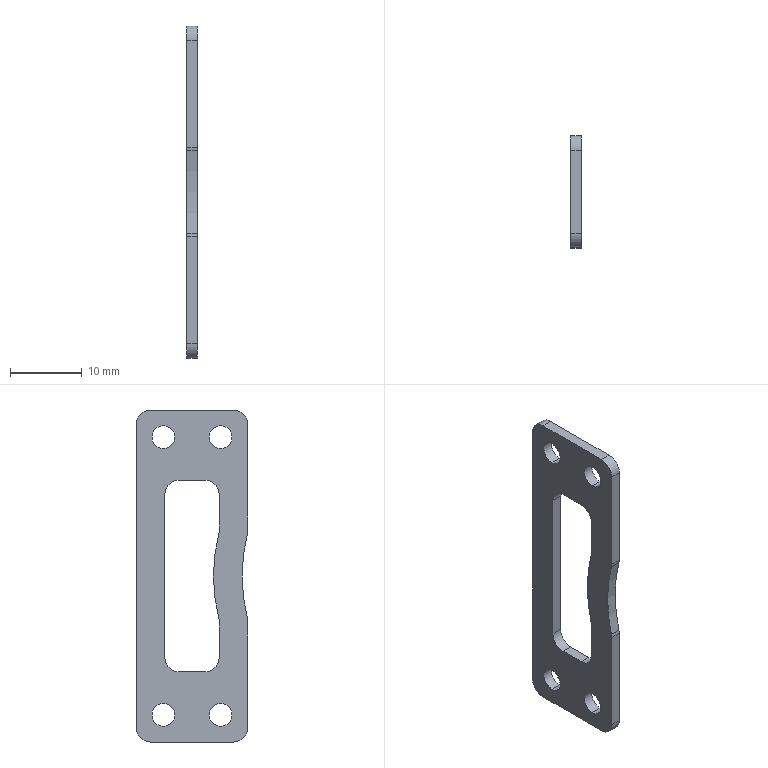Part | SolidWorks | features ICE 2, Extrusion 1, Fillet 1 | 1 solid | 34 faces | box 1.5 x 15.6 x 46.4 mm | volume 731.985 mm3 | cylinder 22 | plane 12 | commonest cylinder face diameters 4 x12 3.2 x8 46 x2
STEP:
#1=CARTESIAN_POINT('',(1.5,-8.,-37.2));
#2=VERTEX_POINT('',#1);
#3=CARTESIAN_POINT('',(1.5,-8.,-40.4));
#4=VERTEX_POINT('',#3);
#5=CARTESIAN_POINT('',(1.5,-8.,-38.8));
#6=DIRECTION('',(1.,0.,0.));
#7=DIRECTION('',(0.,0.,-1.));
#8=AXIS2_PLACEMENT_3D('',#5,#6,#7);
#9=CIRCLE('',#8,1.6);
#10=EDGE_CURVE('',#2,#4,#9,.T.);
#11=ORIENTED_EDGE('',*,*,#10,.T.);
#12=CARTESIAN_POINT('',(0.,-8.,-40.4));
#13=VERTEX_POINT('',#12);
#14=CARTESIAN_POINT('',(1.5,-8.,-40.4));
#15=DIRECTION('',(-1.,0.,0.));
#16=VECTOR('',#15,1000.);
#17=LINE('',#14,#16);
#18=EDGE_CURVE('',#4,#13,#17,.T.);
#19=ORIENTED_EDGE('',*,*,#18,.T.);
#20=CARTESIAN_POINT('',(0.,-8.,-37.2));
#21=VERTEX_POINT('',#20);
#22=CARTESIAN_POINT('',(0.,-8.,-38.8));
#23=DIRECTION('',(1.,0.,0.));
#24=DIRECTION('',(0.,0.,-1.));
#25=AXIS2_PLACEMENT_3D('',#22,#23,#24);
#26=CIRCLE('',#25,1.6);
#27=EDGE_CURVE('',#21,#13,#26,.T.);
#28=ORIENTED_EDGE('',*,*,#27,.F.);
#29=CARTESIAN_POINT('',(1.5,-8.,-37.2));
#30=DIRECTION('',(-1.,0.,0.));
#31=VECTOR('',#30,1000.);
#32=LINE('',#29,#31);
#33=EDGE_CURVE('',#2,#21,#32,.T.);
#34=ORIENTED_EDGE('',*,*,#33,.F.);
#35=EDGE_LOOP('',(#11,#19,#28,#34));
#36=FACE_OUTER_BOUND('',#35,.T.);
#37=CARTESIAN_POINT('',(1.5,-8.,-38.8));
#38=DIRECTION('',(-1.,0.,0.));
#39=DIRECTION('',(0.,0.,1.));
#40=AXIS2_PLACEMENT_3D('',#37,#38,#39);
#41=CYLINDRICAL_SURFACE('',#40,1.6);
#42=ADVANCED_FACE('',(#36),#41,.F.);
#43=CARTESIAN_POINT('',(1.5,0.,-37.2));
#44=VERTEX_POINT('',#43);
#45=CARTESIAN_POINT('',(1.5,0.,-40.4));
#46=VERTEX_POINT('',#45);
#47=CARTESIAN_POINT('',(1.5,0.,-38.8));
#48=DIRECTION('',(1.,0.,0.));
#49=DIRECTION('',(0.,0.,-1.));
#50=AXIS2_PLACEMENT_3D('',#47,#48,#49);
#51=CIRCLE('',#50,1.6);
#52=EDGE_CURVE('',#44,#46,#51,.T.);
#53=ORIENTED_EDGE('',*,*,#52,.T.);
#54=CARTESIAN_POINT('',(0.,0.,-40.4));
#55=VERTEX_POINT('',#54);
#56=CARTESIAN_POINT('',(1.5,0.,-40.4));
#57=DIRECTION('',(-1.,0.,0.));
#58=VECTOR('',#57,1000.);
#59=LINE('',#56,#58);
#60=EDGE_CURVE('',#46,#55,#59,.T.);
#61=ORIENTED_EDGE('',*,*,#60,.T.);
#62=CARTESIAN_POINT('',(0.,0.,-37.2));
#63=VERTEX_POINT('',#62);
#64=CARTESIAN_POINT('',(0.,0.,-38.8));
#65=DIRECTION('',(1.,0.,0.));
#66=DIRECTION('',(0.,0.,-1.));
#67=AXIS2_PLACEMENT_3D('',#64,#65,#66);
#68=CIRCLE('',#67,1.6);
#69=EDGE_CURVE('',#63,#55,#68,.T.);
#70=ORIENTED_EDGE('',*,*,#69,.F.);
#71=CARTESIAN_POINT('',(1.5,0.,-37.2));
#72=DIRECTION('',(-1.,0.,0.));
#73=VECTOR('',#72,1000.);
#74=LINE('',#71,#73);
#75=EDGE_CURVE('',#44,#63,#74,.T.);
#76=ORIENTED_EDGE('',*,*,#75,.F.);
#77=EDGE_LOOP('',(#53,#61,#70,#76));
#78=FACE_OUTER_BOUND('',#77,.T.);
#79=CARTESIAN_POINT('',(1.5,0.,-38.8));
#80=DIRECTION('',(-1.,0.,0.));
#81=DIRECTION('',(0.,0.,1.));
#82=AXIS2_PLACEMENT_3D('',#79,#80,#81);
#83=CYLINDRICAL_SURFACE('',#82,1.6);
#84=ADVANCED_FACE('',(#78),#83,.F.);
#85=CARTESIAN_POINT('',(1.5,-8.,1.6));
#86=VERTEX_POINT('',#85);
#87=CARTESIAN_POINT('',(1.5,-8.,-1.6));
#88=VERTEX_POINT('',#87);
#89=CARTESIAN_POINT('',(1.5,-8.,0.));
#90=DIRECTION('',(1.,0.,0.));
#91=DIRECTION('',(0.,0.,-1.));
#92=AXIS2_PLACEMENT_3D('',#89,#90,#91);
#93=CIRCLE('',#92,1.6);
#94=EDGE_CURVE('',#86,#88,#93,.T.);
#95=ORIENTED_EDGE('',*,*,#94,.T.);
#96=CARTESIAN_POINT('',(0.,-8.,-1.6));
#97=VERTEX_POINT('',#96);
#98=CARTESIAN_POINT('',(1.5,-8.,-1.6));
#99=DIRECTION('',(-1.,0.,0.));
#100=VECTOR('',#99,1000.);
#101=LINE('',#98,#100);
#102=EDGE_CURVE('',#88,#97,#101,.T.);
#103=ORIENTED_EDGE('',*,*,#102,.T.);
#104=CARTESIAN_POINT('',(0.,-8.,1.6));
#105=VERTEX_POINT('',#104);
#106=CARTESIAN_POINT('',(0.,-8.,0.));
#107=DIRECTION('',(1.,0.,0.));
#108=DIRECTION('',(0.,0.,-1.));
#109=AXIS2_PLACEMENT_3D('',#106,#107,#108);
#110=CIRCLE('',#109,1.6);
#111=EDGE_CURVE('',#105,#97,#110,.T.);
#112=ORIENTED_EDGE('',*,*,#111,.F.);
#113=CARTESIAN_POINT('',(1.5,-8.,1.6));
#114=DIRECTION('',(-1.,0.,0.));
#115=VECTOR('',#114,1000.);
#116=LINE('',#113,#115);
#117=EDGE_CURVE('',#86,#105,#116,.T.);
#118=ORIENTED_EDGE('',*,*,#117,.F.);
#119=EDGE_LOOP('',(#95,#103,#112,#118));
#120=FACE_OUTER_BOUND('',#119,.T.);
#121=CARTESIAN_POINT('',(1.5,-8.,0.));
#122=DIRECTION('',(-1.,0.,0.));
#123=DIRECTION('',(0.,0.,1.));
#124=AXIS2_PLACEMENT_3D('',#121,#122,#123);
#125=CYLINDRICAL_SURFACE('',#124,1.6);
#126=ADVANCED_FACE('',(#120),#125,.F.);
#127=CARTESIAN_POINT('',(1.5,0.,1.6));
#128=VERTEX_POINT('',#127);
#129=CARTESIAN_POINT('',(1.5,0.,-1.6));
#130=VERTEX_POINT('',#129);
#131=CARTESIAN_POINT('',(1.5,0.,0.));
#132=DIRECTION('',(1.,0.,0.));
#133=DIRECTION('',(0.,0.,-1.));
#134=AXIS2_PLACEMENT_3D('',#131,#132,#133);
#135=CIRCLE('',#134,1.6);
#136=EDGE_CURVE('',#128,#130,#135,.T.);
#137=ORIENTED_EDGE('',*,*,#136,.T.);
#138=CARTESIAN_POINT('',(0.,0.,-1.6));
#139=VERTEX_POINT('',#138);
#140=CARTESIAN_POINT('',(1.5,0.,-1.6));
#141=DIRECTION('',(-1.,0.,0.));
#142=VECTOR('',#141,1000.);
#143=LINE('',#140,#142);
#144=EDGE_CURVE('',#130,#139,#143,.T.);
#145=ORIENTED_EDGE('',*,*,#144,.T.);
#146=CARTESIAN_POINT('',(0.,0.,1.6));
#147=VERTEX_POINT('',#146);
#148=CARTESIAN_POINT('',(0.,0.,0.));
#149=DIRECTION('',(1.,0.,0.));
#150=DIRECTION('',(0.,0.,-1.));
#151=AXIS2_PLACEMENT_3D('',#148,#149,#150);
#152=CIRCLE('',#151,1.6);
#153=EDGE_CURVE('',#147,#139,#152,.T.);
#154=ORIENTED_EDGE('',*,*,#153,.F.);
#155=CARTESIAN_POINT('',(1.5,0.,1.6));
#156=DIRECTION('',(-1.,0.,0.));
#157=VECTOR('',#156,1000.);
#158=LINE('',#155,#157);
#159=EDGE_CURVE('',#128,#147,#158,.T.);
#160=ORIENTED_EDGE('',*,*,#159,.F.);
#161=EDGE_LOOP('',(#137,#145,#154,#160));
#162=FACE_OUTER_BOUND('',#161,.T.);
#163=CARTESIAN_POINT('',(1.5,0.,0.));
#164=DIRECTION('',(-1.,0.,0.));
#165=DIRECTION('',(0.,0.,1.));
#166=AXIS2_PLACEMENT_3D('',#163,#164,#165);
#167=CYLINDRICAL_SURFACE('',#166,1.6);
#168=ADVANCED_FACE('',(#162),#167,.F.);
#169=CARTESIAN_POINT('',(1.5,-11.8,1.8));
#170=VERTEX_POINT('',#169);
#171=CARTESIAN_POINT('',(1.5,-11.8,-13.126));
#172=VERTEX_POINT('',#171);
#173=CARTESIAN_POINT('',(1.5,-11.8,3.8));
#174=DIRECTION('',(0.,0.,-1.));
#175=VECTOR('',#174,1000.);
#176=LINE('',#173,#175);
#177=EDGE_CURVE('',#170,#172,#176,.T.);
#178=ORIENTED_EDGE('',*,*,#177,.F.);
#179=CARTESIAN_POINT('',(0.,-11.8,1.8));
#180=VERTEX_POINT('',#179);
#181=CARTESIAN_POINT('',(1.5,-11.8,1.8));
#182=DIRECTION('',(-1.,0.,0.));
#183=VECTOR('',#182,1000.);
#184=LINE('',#181,#183);
#185=EDGE_CURVE('',#170,#180,#184,.T.);
#186=ORIENTED_EDGE('',*,*,#185,.T.);
#187=CARTESIAN_POINT('',(0.,-11.8,-13.126));
#188=VERTEX_POINT('',#187);
#189=CARTESIAN_POINT('',(0.,-11.8,3.8));
#190=DIRECTION('',(0.,0.,-1.));
#191=VECTOR('',#190,1000.);
#192=LINE('',#189,#191);
#193=EDGE_CURVE('',#180,#188,#192,.T.);
#194=ORIENTED_EDGE('',*,*,#193,.T.);
#195=CARTESIAN_POINT('',(1.5,-11.8,-13.126));
#196=DIRECTION('',(1.,0.,0.));
#197=VECTOR('',#196,1000.);
#198=LINE('',#195,#197);
#199=EDGE_CURVE('',#188,#172,#198,.T.);
#200=ORIENTED_EDGE('',*,*,#199,.T.);
#201=EDGE_LOOP('',(#178,#186,#194,#200));
#202=FACE_OUTER_BOUND('',#201,.T.);
#203=CARTESIAN_POINT('',(1.5,-11.8,3.8));
#204=DIRECTION('',(0.,1.,0.));
#205=DIRECTION('',(0.,0.,1.));
#206=AXIS2_PLACEMENT_3D('',#203,#204,#205);
#207=PLANE('',#206);
#208=ADVANCED_FACE('',(#202),#207,.F.);
#209=CARTESIAN_POINT('',(1.5,-2.2,-6.));
#210=VERTEX_POINT('',#209);
#211=CARTESIAN_POINT('',(1.5,-5.8,-6.));
#212=VERTEX_POINT('',#211);
#213=CARTESIAN_POINT('',(1.5,-0.2,-6.));
#214=DIRECTION('',(0.,-1.,0.));
#215=VECTOR('',#214,1000.);
#216=LINE('',#213,#215);
#217=EDGE_CURVE('',#210,#212,#216,.T.);
#218=ORIENTED_EDGE('',*,*,#217,.F.);
#219=CARTESIAN_POINT('',(1.5,-0.2,-8.));
#220=VERTEX_POINT('',#219);
#221=CARTESIAN_POINT('',(1.5,-2.2,-8.));
#222=DIRECTION('',(-1.,0.,0.));
#223=DIRECTION('',(0.,0.,-1.));
#224=AXIS2_PLACEMENT_3D('',#221,#222,#223);
#225=CIRCLE('',#224,2.);
#226=EDGE_CURVE('',#210,#220,#225,.T.);
#227=ORIENTED_EDGE('',*,*,#226,.T.);
#228=CARTESIAN_POINT('',(1.5,-0.2,-30.8));
#229=VERTEX_POINT('',#228);
#230=CARTESIAN_POINT('',(1.5,-0.2,-6.));
#231=DIRECTION('',(0.,0.,1.));
#232=VECTOR('',#231,1000.);
#233=LINE('',#230,#232);
#234=EDGE_CURVE('',#229,#220,#233,.T.);
#235=ORIENTED_EDGE('',*,*,#234,.F.);
#236=CARTESIAN_POINT('',(1.5,-2.2,-32.8));
#237=VERTEX_POINT('',#236);
#238=CARTESIAN_POINT('',(1.5,-2.2,-30.8));
#239=DIRECTION('',(-1.,0.,0.));
#240=DIRECTION('',(0.,0.,-1.));
#241=AXIS2_PLACEMENT_3D('',#238,#239,#240);
#242=CIRCLE('',#241,2.);
#243=EDGE_CURVE('',#229,#237,#242,.T.);
#244=ORIENTED_EDGE('',*,*,#243,.T.);
#245=CARTESIAN_POINT('',(1.5,-5.8,-32.8));
#246=VERTEX_POINT('',#245);
#247=CARTESIAN_POINT('',(1.5,-0.2,-32.8));
#248=DIRECTION('',(0.,1.,0.));
#249=VECTOR('',#248,1000.);
#250=LINE('',#247,#249);
#251=EDGE_CURVE('',#246,#237,#250,.T.);
#252=ORIENTED_EDGE('',*,*,#251,.F.);
#253=CARTESIAN_POINT('',(1.5,-7.8,-30.8));
#254=VERTEX_POINT('',#253);
#255=CARTESIAN_POINT('',(1.5,-5.8,-30.8));
#256=DIRECTION('',(-1.,0.,0.));
#257=DIRECTION('',(0.,0.,-1.));
#258=AXIS2_PLACEMENT_3D('',#255,#256,#257);
#259=CIRCLE('',#258,2.);
#260=EDGE_CURVE('',#246,#254,#259,.T.);
#261=ORIENTED_EDGE('',*,*,#260,.T.);
#262=CARTESIAN_POINT('',(1.5,-7.8,-25.674));
#263=VERTEX_POINT('',#262);
#264=CARTESIAN_POINT('',(1.5,-7.8,-25.413));
#265=DIRECTION('',(0.,0.,-1.));
#266=VECTOR('',#265,1000.);
#267=LINE('',#264,#266);
#268=EDGE_CURVE('',#263,#254,#267,.T.);
#269=ORIENTED_EDGE('',*,*,#268,.F.);
#270=CARTESIAN_POINT('',(1.5,-7.736,-25.172));
#271=VERTEX_POINT('',#270);
#272=CARTESIAN_POINT('',(1.5,-5.8,-25.674));
#273=DIRECTION('',(-1.,0.,0.));
#274=DIRECTION('',(0.,0.,-1.));
#275=AXIS2_PLACEMENT_3D('',#272,#273,#274);
#276=CIRCLE('',#275,2.);
#277=EDGE_CURVE('',#263,#271,#276,.T.);
#278=ORIENTED_EDGE('',*,*,#277,.T.);
#279=CARTESIAN_POINT('',(1.5,-7.736,-13.628));
#280=VERTEX_POINT('',#279);
#281=CARTESIAN_POINT('',(1.5,-30.,-19.4));
#282=DIRECTION('',(-1.,0.,0.));
#283=DIRECTION('',(0.,0.,-1.));
#284=AXIS2_PLACEMENT_3D('',#281,#282,#283);
#285=CIRCLE('',#284,23.);
#286=EDGE_CURVE('',#280,#271,#285,.T.);
#287=ORIENTED_EDGE('',*,*,#286,.F.);
#288=CARTESIAN_POINT('',(1.5,-7.8,-13.126));
#289=VERTEX_POINT('',#288);
#290=CARTESIAN_POINT('',(1.5,-5.8,-13.126));
#291=DIRECTION('',(-1.,0.,0.));
#292=DIRECTION('',(0.,0.,-1.));
#293=AXIS2_PLACEMENT_3D('',#290,#291,#292);
#294=CIRCLE('',#293,2.);
#295=EDGE_CURVE('',#280,#289,#294,.T.);
#296=ORIENTED_EDGE('',*,*,#295,.T.);
#297=CARTESIAN_POINT('',(1.5,-7.8,-8.));
#298=VERTEX_POINT('',#297);
#299=CARTESIAN_POINT('',(1.5,-7.8,-6.));
#300=DIRECTION('',(0.,0.,-1.));
#301=VECTOR('',#300,1000.);
#302=LINE('',#299,#301);
#303=EDGE_CURVE('',#298,#289,#302,.T.);
#304=ORIENTED_EDGE('',*,*,#303,.F.);
#305=CARTESIAN_POINT('',(1.5,-5.8,-8.));
#306=DIRECTION('',(-1.,0.,0.));
#307=DIRECTION('',(0.,0.,-1.));
#308=AXIS2_PLACEMENT_3D('',#305,#306,#307);
#309=CIRCLE('',#308,2.);
#310=EDGE_CURVE('',#298,#212,#309,.T.);
#311=ORIENTED_EDGE('',*,*,#310,.T.);
#312=EDGE_LOOP('',(#218,#227,#235,#244,#252,#261,#269,#278,#287,#296,#304,#311));
#313=FACE_BOUND('',#312,.T.);
#314=CARTESIAN_POINT('',(1.5,-11.8,-25.674));
#315=VERTEX_POINT('',#314);
#316=CARTESIAN_POINT('',(1.5,-11.8,-40.6));
#317=VERTEX_POINT('',#316);
#318=CARTESIAN_POINT('',(1.5,-11.8,3.8));
#319=DIRECTION('',(0.,0.,-1.));
#320=VECTOR('',#319,1000.);
#321=LINE('',#318,#320);
#322=EDGE_CURVE('',#315,#317,#321,.T.);
#323=ORIENTED_EDGE('',*,*,#322,.T.);
#324=CARTESIAN_POINT('',(1.5,-9.8,-42.6));
#325=VERTEX_POINT('',#324);
#326=CARTESIAN_POINT('',(1.5,-9.8,-40.6));
#327=DIRECTION('',(1.,0.,0.));
#328=DIRECTION('',(0.,0.,-1.));
#329=AXIS2_PLACEMENT_3D('',#326,#327,#328);
#330=CIRCLE('',#329,2.);
#331=EDGE_CURVE('',#317,#325,#330,.T.);
#332=ORIENTED_EDGE('',*,*,#331,.T.);
#333=CARTESIAN_POINT('',(1.5,1.8,-42.6));
#334=VERTEX_POINT('',#333);
#335=CARTESIAN_POINT('',(1.5,3.8,-42.6));
#336=DIRECTION('',(0.,1.,0.));
#337=VECTOR('',#336,1000.);
#338=LINE('',#335,#337);
#339=EDGE_CURVE('',#325,#334,#338,.T.);
#340=ORIENTED_EDGE('',*,*,#339,.T.);
#341=CARTESIAN_POINT('',(1.5,3.8,-40.6));
#342=VERTEX_POINT('',#341);
#343=CARTESIAN_POINT('',(1.5,1.8,-40.6));
#344=DIRECTION('',(1.,0.,0.));
#345=DIRECTION('',(0.,0.,-1.));
#346=AXIS2_PLACEMENT_3D('',#343,#344,#345);
#347=CIRCLE('',#346,2.);
#348=EDGE_CURVE('',#334,#342,#347,.T.);
#349=ORIENTED_EDGE('',*,*,#348,.T.);
#350=CARTESIAN_POINT('',(1.5,3.8,1.8));
#351=VERTEX_POINT('',#350);
#352=CARTESIAN_POINT('',(1.5,3.8,3.8));
#353=DIRECTION('',(0.,0.,1.));
#354=VECTOR('',#353,1000.);
#355=LINE('',#352,#354);
#356=EDGE_CURVE('',#342,#351,#355,.T.);
#357=ORIENTED_EDGE('',*,*,#356,.T.);
#358=CARTESIAN_POINT('',(1.5,1.8,3.8));
#359=VERTEX_POINT('',#358);
#360=CARTESIAN_POINT('',(1.5,1.8,1.8));
#361=DIRECTION('',(1.,0.,0.));
#362=DIRECTION('',(0.,0.,-1.));
#363=AXIS2_PLACEMENT_3D('',#360,#361,#362);
#364=CIRCLE('',#363,2.);
#365=EDGE_CURVE('',#351,#359,#364,.T.);
#366=ORIENTED_EDGE('',*,*,#365,.T.);
#367=CARTESIAN_POINT('',(1.5,-9.8,3.8));
#368=VERTEX_POINT('',#367);
#369=CARTESIAN_POINT('',(1.5,3.8,3.8));
#370=DIRECTION('',(0.,-1.,0.));
#371=VECTOR('',#370,1000.);
#372=LINE('',#369,#371);
#373=EDGE_CURVE('',#359,#368,#372,.T.);
#374=ORIENTED_EDGE('',*,*,#373,.T.);
#375=CARTESIAN_POINT('',(1.5,-9.8,1.8));
#376=DIRECTION('',(1.,0.,0.));
#377=DIRECTION('',(0.,0.,-1.));
#378=AXIS2_PLACEMENT_3D('',#375,#376,#377);
#379=CIRCLE('',#378,2.);
#380=EDGE_CURVE('',#368,#170,#379,.T.);
#381=ORIENTED_EDGE('',*,*,#380,.T.);
#382=ORIENTED_EDGE('',*,*,#177,.T.);
#383=CARTESIAN_POINT('',(1.5,-11.736,-13.628));
#384=VERTEX_POINT('',#383);
#385=CARTESIAN_POINT('',(1.5,-9.8,-13.126));
#386=DIRECTION('',(1.,0.,0.));
#387=DIRECTION('',(0.,0.,-1.));
#388=AXIS2_PLACEMENT_3D('',#385,#386,#387);
#389=CIRCLE('',#388,2.);
#390=EDGE_CURVE('',#172,#384,#389,.T.);
#391=ORIENTED_EDGE('',*,*,#390,.T.);
#392=CARTESIAN_POINT('',(1.5,-11.736,-25.172));
#393=VERTEX_POINT('',#392);
#394=CARTESIAN_POINT('',(1.5,-34.,-19.4));
#395=DIRECTION('',(1.,0.,0.));
#396=DIRECTION('',(0.,0.,-1.));
#397=AXIS2_PLACEMENT_3D('',#394,#395,#396);
#398=CIRCLE('',#397,23.);
#399=EDGE_CURVE('',#393,#384,#398,.T.);
#400=ORIENTED_EDGE('',*,*,#399,.F.);
#401=CARTESIAN_POINT('',(1.5,-9.8,-25.674));
#402=DIRECTION('',(1.,0.,0.));
#403=DIRECTION('',(0.,0.,-1.));
#404=AXIS2_PLACEMENT_3D('',#401,#402,#403);
#405=CIRCLE('',#404,2.);
#406=EDGE_CURVE('',#393,#315,#405,.T.);
#407=ORIENTED_EDGE('',*,*,#406,.T.);
#408=EDGE_LOOP('',(#323,#332,#340,#349,#357,#366,#374,#381,#382,#391,#400,#407));
#409=FACE_OUTER_BOUND('',#408,.T.);
#410=ORIENTED_EDGE('',*,*,#52,.F.);
#411=CARTESIAN_POINT('',(1.5,0.,-38.8));
#412=DIRECTION('',(1.,0.,0.));
#413=DIRECTION('',(0.,0.,-1.));
#414=AXIS2_PLACEMENT_3D('',#411,#412,#413);
#415=CIRCLE('',#414,1.6);
#416=EDGE_CURVE('',#46,#44,#415,.T.);
#417=ORIENTED_EDGE('',*,*,#416,.F.);
#418=EDGE_LOOP('',(#410,#417));
#419=FACE_BOUND('',#418,.T.);
#420=ORIENTED_EDGE('',*,*,#136,.F.);
#421=CARTESIAN_POINT('',(1.5,0.,0.));
#422=DIRECTION('',(1.,0.,0.));
#423=DIRECTION('',(0.,0.,-1.));
#424=AXIS2_PLACEMENT_3D('',#421,#422,#423);
#425=CIRCLE('',#424,1.6);
#426=EDGE_CURVE('',#130,#128,#425,.T.);
#427=ORIENTED_EDGE('',*,*,#426,.F.);
#428=EDGE_LOOP('',(#420,#427));
#429=FACE_BOUND('',#428,.T.);
#430=ORIENTED_EDGE('',*,*,#94,.F.);
#431=CARTESIAN_POINT('',(1.5,-8.,0.));
#432=DIRECTION('',(1.,0.,0.));
#433=DIRECTION('',(0.,0.,-1.));
#434=AXIS2_PLACEMENT_3D('',#431,#432,#433);
#435=CIRCLE('',#434,1.6);
#436=EDGE_CURVE('',#88,#86,#435,.T.);
#437=ORIENTED_EDGE('',*,*,#436,.F.);
#438=EDGE_LOOP('',(#430,#437));
#439=FACE_BOUND('',#438,.T.);
#440=ORIENTED_EDGE('',*,*,#10,.F.);
#441=CARTESIAN_POINT('',(1.5,-8.,-38.8));
#442=DIRECTION('',(1.,0.,0.));
#443=DIRECTION('',(0.,0.,-1.));
#444=AXIS2_PLACEMENT_3D('',#441,#442,#443);
#445=CIRCLE('',#444,1.6);
#446=EDGE_CURVE('',#4,#2,#445,.T.);
#447=ORIENTED_EDGE('',*,*,#446,.F.);
#448=EDGE_LOOP('',(#440,#447));
#449=FACE_BOUND('',#448,.T.);
#450=CARTESIAN_POINT('',(1.5,0.,0.));
#451=DIRECTION('',(1.,0.,0.));
#452=DIRECTION('',(0.,0.,-1.));
#453=AXIS2_PLACEMENT_3D('',#450,#451,#452);
#454=PLANE('',#453);
#455=ADVANCED_FACE('',(#313,#409,#419,#429,#439,#449),#454,.T.);
#456=CARTESIAN_POINT('',(0.,-5.8,-32.8));
#457=VERTEX_POINT('',#456);
#458=CARTESIAN_POINT('',(0.,-2.2,-32.8));
#459=VERTEX_POINT('',#458);
#460=CARTESIAN_POINT('',(0.,-0.2,-32.8));
#461=DIRECTION('',(0.,1.,0.));
#462=VECTOR('',#461,1000.);
#463=LINE('',#460,#462);
#464=EDGE_CURVE('',#457,#459,#463,.T.);
#465=ORIENTED_EDGE('',*,*,#464,.T.);
#466=CARTESIAN_POINT('',(0.,-0.2,-30.8));
#467=VERTEX_POINT('',#466);
#468=CARTESIAN_POINT('',(0.,-2.2,-30.8));
#469=DIRECTION('',(1.,0.,0.));
#470=DIRECTION('',(0.,0.,-1.));
#471=AXIS2_PLACEMENT_3D('',#468,#469,#470);
#472=CIRCLE('',#471,2.);
#473=EDGE_CURVE('',#459,#467,#472,.T.);
#474=ORIENTED_EDGE('',*,*,#473,.T.);
#475=CARTESIAN_POINT('',(0.,-0.2,-8.));
#476=VERTEX_POINT('',#475);
#477=CARTESIAN_POINT('',(0.,-0.2,-6.));
#478=DIRECTION('',(0.,0.,1.));
#479=VECTOR('',#478,1000.);
#480=LINE('',#477,#479);
#481=EDGE_CURVE('',#467,#476,#480,.T.);
#482=ORIENTED_EDGE('',*,*,#481,.T.);
#483=CARTESIAN_POINT('',(0.,-2.2,-6.));
#484=VERTEX_POINT('',#483);
#485=CARTESIAN_POINT('',(0.,-2.2,-8.));
#486=DIRECTION('',(1.,0.,0.));
#487=DIRECTION('',(0.,0.,-1.));
#488=AXIS2_PLACEMENT_3D('',#485,#486,#487);
#489=CIRCLE('',#488,2.);
#490=EDGE_CURVE('',#476,#484,#489,.T.);
#491=ORIENTED_EDGE('',*,*,#490,.T.);
#492=CARTESIAN_POINT('',(0.,-5.8,-6.));
#493=VERTEX_POINT('',#492);
#494=CARTESIAN_POINT('',(0.,-0.2,-6.));
#495=DIRECTION('',(0.,-1.,0.));
#496=VECTOR('',#495,1000.);
#497=LINE('',#494,#496);
#498=EDGE_CURVE('',#484,#493,#497,.T.);
#499=ORIENTED_EDGE('',*,*,#498,.T.);
#500=CARTESIAN_POINT('',(0.,-7.8,-8.));
#501=VERTEX_POINT('',#500);
#502=CARTESIAN_POINT('',(0.,-5.8,-8.));
#503=DIRECTION('',(1.,0.,0.));
#504=DIRECTION('',(0.,0.,-1.));
#505=AXIS2_PLACEMENT_3D('',#502,#503,#504);
#506=CIRCLE('',#505,2.);
#507=EDGE_CURVE('',#493,#501,#506,.T.);
#508=ORIENTED_EDGE('',*,*,#507,.T.);
#509=CARTESIAN_POINT('',(0.,-7.8,-13.126));
#510=VERTEX_POINT('',#509);
#511=CARTESIAN_POINT('',(0.,-7.8,-6.));
#512=DIRECTION('',(0.,0.,-1.));
#513=VECTOR('',#512,1000.);
#514=LINE('',#511,#513);
#515=EDGE_CURVE('',#501,#510,#514,.T.);
#516=ORIENTED_EDGE('',*,*,#515,.T.);
#517=CARTESIAN_POINT('',(0.,-7.736,-13.628));
#518=VERTEX_POINT('',#517);
#519=CARTESIAN_POINT('',(0.,-5.8,-13.126));
#520=DIRECTION('',(1.,0.,0.));
#521=DIRECTION('',(0.,0.,-1.));
#522=AXIS2_PLACEMENT_3D('',#519,#520,#521);
#523=CIRCLE('',#522,2.);
#524=EDGE_CURVE('',#510,#518,#523,.T.);
#525=ORIENTED_EDGE('',*,*,#524,.T.);
#526=CARTESIAN_POINT('',(0.,-7.736,-25.172));
#527=VERTEX_POINT('',#526);
#528=CARTESIAN_POINT('',(0.,-30.,-19.4));
#529=DIRECTION('',(-1.,0.,0.));
#530=DIRECTION('',(0.,0.,-1.));
#531=AXIS2_PLACEMENT_3D('',#528,#529,#530);
#532=CIRCLE('',#531,23.);
#533=EDGE_CURVE('',#518,#527,#532,.T.);
#534=ORIENTED_EDGE('',*,*,#533,.T.);
#535=CARTESIAN_POINT('',(0.,-7.8,-25.674));
#536=VERTEX_POINT('',#535);
#537=CARTESIAN_POINT('',(0.,-5.8,-25.674));
#538=DIRECTION('',(1.,0.,0.));
#539=DIRECTION('',(0.,0.,-1.));
#540=AXIS2_PLACEMENT_3D('',#537,#538,#539);
#541=CIRCLE('',#540,2.);
#542=EDGE_CURVE('',#527,#536,#541,.T.);
#543=ORIENTED_EDGE('',*,*,#542,.T.);
#544=CARTESIAN_POINT('',(0.,-7.8,-30.8));
#545=VERTEX_POINT('',#544);
#546=CARTESIAN_POINT('',(0.,-7.8,-25.413));
#547=DIRECTION('',(0.,0.,-1.));
#548=VECTOR('',#547,1000.);
#549=LINE('',#546,#548);
#550=EDGE_CURVE('',#536,#545,#549,.T.);
#551=ORIENTED_EDGE('',*,*,#550,.T.);
#552=CARTESIAN_POINT('',(0.,-5.8,-30.8));
#553=DIRECTION('',(1.,0.,0.));
#554=DIRECTION('',(0.,0.,-1.));
#555=AXIS2_PLACEMENT_3D('',#552,#553,#554);
#556=CIRCLE('',#555,2.);
#557=EDGE_CURVE('',#545,#457,#556,.T.);
#558=ORIENTED_EDGE('',*,*,#557,.T.);
#559=EDGE_LOOP('',(#465,#474,#482,#491,#499,#508,#516,#525,#534,#543,#551,#558));
#560=FACE_BOUND('',#559,.T.);
#561=CARTESIAN_POINT('',(0.,-9.8,-42.6));
#562=VERTEX_POINT('',#561);
#563=CARTESIAN_POINT('',(0.,1.8,-42.6));
#564=VERTEX_POINT('',#563);
#565=CARTESIAN_POINT('',(0.,3.8,-42.6));
#566=DIRECTION('',(0.,1.,0.));
#567=VECTOR('',#566,1000.);
#568=LINE('',#565,#567);
#569=EDGE_CURVE('',#562,#564,#568,.T.);
#570=ORIENTED_EDGE('',*,*,#569,.F.);
#571=CARTESIAN_POINT('',(0.,-11.8,-40.6));
#572=VERTEX_POINT('',#571);
#573=CARTESIAN_POINT('',(0.,-9.8,-40.6));
#574=DIRECTION('',(-1.,0.,0.));
#575=DIRECTION('',(0.,0.,-1.));
#576=AXIS2_PLACEMENT_3D('',#573,#574,#575);
#577=CIRCLE('',#576,2.);
#578=EDGE_CURVE('',#562,#572,#577,.T.);
#579=ORIENTED_EDGE('',*,*,#578,.T.);
#580=CARTESIAN_POINT('',(0.,-11.8,-25.674));
#581=VERTEX_POINT('',#580);
#582=CARTESIAN_POINT('',(0.,-11.8,3.8));
#583=DIRECTION('',(0.,0.,-1.));
#584=VECTOR('',#583,1000.);
#585=LINE('',#582,#584);
#586=EDGE_CURVE('',#581,#572,#585,.T.);
#587=ORIENTED_EDGE('',*,*,#586,.F.);
#588=CARTESIAN_POINT('',(0.,-11.736,-25.172));
#589=VERTEX_POINT('',#588);
#590=CARTESIAN_POINT('',(0.,-9.8,-25.674));
#591=DIRECTION('',(-1.,0.,0.));
#592=DIRECTION('',(0.,0.,-1.));
#593=AXIS2_PLACEMENT_3D('',#590,#591,#592);
#594=CIRCLE('',#593,2.);
#595=EDGE_CURVE('',#581,#589,#594,.T.);
#596=ORIENTED_EDGE('',*,*,#595,.T.);
#597=CARTESIAN_POINT('',(0.,-11.736,-13.628));
#598=VERTEX_POINT('',#597);
#599=CARTESIAN_POINT('',(0.,-34.,-19.4));
#600=DIRECTION('',(1.,0.,0.));
#601=DIRECTION('',(0.,0.,-1.));
#602=AXIS2_PLACEMENT_3D('',#599,#600,#601);
#603=CIRCLE('',#602,23.);
#604=EDGE_CURVE('',#589,#598,#603,.T.);
#605=ORIENTED_EDGE('',*,*,#604,.T.);
#606=CARTESIAN_POINT('',(0.,-9.8,-13.126));
#607=DIRECTION('',(-1.,0.,0.));
#608=DIRECTION('',(0.,0.,-1.));
#609=AXIS2_PLACEMENT_3D('',#606,#607,#608);
#610=CIRCLE('',#609,2.);
#611=EDGE_CURVE('',#598,#188,#610,.T.);
#612=ORIENTED_EDGE('',*,*,#611,.T.);
#613=ORIENTED_EDGE('',*,*,#193,.F.);
#614=CARTESIAN_POINT('',(0.,-9.8,3.8));
#615=VERTEX_POINT('',#614);
#616=CARTESIAN_POINT('',(0.,-9.8,1.8));
#617=DIRECTION('',(-1.,0.,0.));
#618=DIRECTION('',(0.,0.,-1.));
#619=AXIS2_PLACEMENT_3D('',#616,#617,#618);
#620=CIRCLE('',#619,2.);
#621=EDGE_CURVE('',#180,#615,#620,.T.);
#622=ORIENTED_EDGE('',*,*,#621,.T.);
#623=CARTESIAN_POINT('',(0.,1.8,3.8));
#624=VERTEX_POINT('',#623);
#625=CARTESIAN_POINT('',(0.,3.8,3.8));
#626=DIRECTION('',(0.,-1.,0.));
#627=VECTOR('',#626,1000.);
#628=LINE('',#625,#627);
#629=EDGE_CURVE('',#624,#615,#628,.T.);
#630=ORIENTED_EDGE('',*,*,#629,.F.);
#631=CARTESIAN_POINT('',(0.,3.8,1.8));
#632=VERTEX_POINT('',#631);
#633=CARTESIAN_POINT('',(0.,1.8,1.8));
#634=DIRECTION('',(-1.,0.,0.));
#635=DIRECTION('',(0.,0.,-1.));
#636=AXIS2_PLACEMENT_3D('',#633,#634,#635);
#637=CIRCLE('',#636,2.);
#638=EDGE_CURVE('',#624,#632,#637,.T.);
#639=ORIENTED_EDGE('',*,*,#638,.T.);
#640=CARTESIAN_POINT('',(0.,3.8,-40.6));
#641=VERTEX_POINT('',#640);
#642=CARTESIAN_POINT('',(0.,3.8,3.8));
#643=DIRECTION('',(0.,0.,1.));
#644=VECTOR('',#643,1000.);
#645=LINE('',#642,#644);
#646=EDGE_CURVE('',#641,#632,#645,.T.);
#647=ORIENTED_EDGE('',*,*,#646,.F.);
#648=CARTESIAN_POINT('',(0.,1.8,-40.6));
#649=DIRECTION('',(-1.,0.,0.));
#650=DIRECTION('',(0.,0.,-1.));
#651=AXIS2_PLACEMENT_3D('',#648,#649,#650);
#652=CIRCLE('',#651,2.);
#653=EDGE_CURVE('',#641,#564,#652,.T.);
#654=ORIENTED_EDGE('',*,*,#653,.T.);
#655=EDGE_LOOP('',(#570,#579,#587,#596,#605,#612,#613,#622,#630,#639,#647,#654));
#656=FACE_OUTER_BOUND('',#655,.T.);
#657=ORIENTED_EDGE('',*,*,#153,.T.);
#658=CARTESIAN_POINT('',(0.,0.,0.));
#659=DIRECTION('',(1.,0.,0.));
#660=DIRECTION('',(0.,0.,-1.));
#661=AXIS2_PLACEMENT_3D('',#658,#659,#660);
#662=CIRCLE('',#661,1.6);
#663=EDGE_CURVE('',#139,#147,#662,.T.);
#664=ORIENTED_EDGE('',*,*,#663,.T.);
#665=EDGE_LOOP('',(#657,#664));
#666=FACE_BOUND('',#665,.T.);
#667=ORIENTED_EDGE('',*,*,#111,.T.);
#668=CARTESIAN_POINT('',(0.,-8.,0.));
#669=DIRECTION('',(1.,0.,0.));
#670=DIRECTION('',(0.,0.,-1.));
#671=AXIS2_PLACEMENT_3D('',#668,#669,#670);
#672=CIRCLE('',#671,1.6);
#673=EDGE_CURVE('',#97,#105,#672,.T.);
#674=ORIENTED_EDGE('',*,*,#673,.T.);
#675=EDGE_LOOP('',(#667,#674));
#676=FACE_BOUND('',#675,.T.);
#677=ORIENTED_EDGE('',*,*,#69,.T.);
#678=CARTESIAN_POINT('',(0.,0.,-38.8));
#679=DIRECTION('',(1.,0.,0.));
#680=DIRECTION('',(0.,0.,-1.));
#681=AXIS2_PLACEMENT_3D('',#678,#679,#680);
#682=CIRCLE('',#681,1.6);
#683=EDGE_CURVE('',#55,#63,#682,.T.);
#684=ORIENTED_EDGE('',*,*,#683,.T.);
#685=EDGE_LOOP('',(#677,#684));
#686=FACE_BOUND('',#685,.T.);
#687=ORIENTED_EDGE('',*,*,#27,.T.);
#688=CARTESIAN_POINT('',(0.,-8.,-38.8));
#689=DIRECTION('',(1.,0.,0.));
#690=DIRECTION('',(0.,0.,-1.));
#691=AXIS2_PLACEMENT_3D('',#688,#689,#690);
#692=CIRCLE('',#691,1.6);
#693=EDGE_CURVE('',#13,#21,#692,.T.);
#694=ORIENTED_EDGE('',*,*,#693,.T.);
#695=EDGE_LOOP('',(#687,#694));
#696=FACE_BOUND('',#695,.T.);
#697=CARTESIAN_POINT('',(0.,0.,0.));
#698=DIRECTION('',(1.,0.,0.));
#699=DIRECTION('',(0.,0.,-1.));
#700=AXIS2_PLACEMENT_3D('',#697,#698,#699);
#701=PLANE('',#700);
#702=ADVANCED_FACE('',(#560,#656,#666,#676,#686,#696),#701,.F.);
#703=ORIENTED_EDGE('',*,*,#373,.F.);
#704=CARTESIAN_POINT('',(1.5,1.8,3.8));
#705=DIRECTION('',(-1.,0.,0.));
#706=VECTOR('',#705,1000.);
#707=LINE('',#704,#706);
#708=EDGE_CURVE('',#359,#624,#707,.T.);
#709=ORIENTED_EDGE('',*,*,#708,.T.);
#710=ORIENTED_EDGE('',*,*,#629,.T.);
#711=CARTESIAN_POINT('',(1.5,-9.8,3.8));
#712=DIRECTION('',(1.,0.,0.));
#713=VECTOR('',#712,1000.);
#714=LINE('',#711,#713);
#715=EDGE_CURVE('',#615,#368,#714,.T.);
#716=ORIENTED_EDGE('',*,*,#715,.T.);
#717=EDGE_LOOP('',(#703,#709,#710,#716));
#718=FACE_OUTER_BOUND('',#717,.T.);
#719=CARTESIAN_POINT('',(1.5,3.8,3.8));
#720=DIRECTION('',(0.,0.,-1.));
#721=DIRECTION('',(0.,1.,0.));
#722=AXIS2_PLACEMENT_3D('',#719,#720,#721);
#723=PLANE('',#722);
#724=ADVANCED_FACE('',(#718),#723,.F.);
#725=ORIENTED_EDGE('',*,*,#586,.T.);
#726=CARTESIAN_POINT('',(1.5,-11.8,-40.6));
#727=DIRECTION('',(1.,0.,0.));
#728=VECTOR('',#727,1000.);
#729=LINE('',#726,#728);
#730=EDGE_CURVE('',#572,#317,#729,.T.);
#731=ORIENTED_EDGE('',*,*,#730,.T.);
#732=ORIENTED_EDGE('',*,*,#322,.F.);
#733=CARTESIAN_POINT('',(1.5,-11.8,-25.674));
#734=DIRECTION('',(-1.,0.,0.));
#735=VECTOR('',#734,1000.);
#736=LINE('',#733,#735);
#737=EDGE_CURVE('',#315,#581,#736,.T.);
#738=ORIENTED_EDGE('',*,*,#737,.T.);
#739=EDGE_LOOP('',(#725,#731,#732,#738));
#740=FACE_OUTER_BOUND('',#739,.T.);
#741=CARTESIAN_POINT('',(1.5,-11.8,3.8));
#742=DIRECTION('',(0.,1.,0.));
#743=DIRECTION('',(0.,0.,1.));
#744=AXIS2_PLACEMENT_3D('',#741,#742,#743);
#745=PLANE('',#744);
#746=ADVANCED_FACE('',(#740),#745,.F.);
#747=ORIENTED_EDGE('',*,*,#339,.F.);
#748=CARTESIAN_POINT('',(1.5,-9.8,-42.6));
#749=DIRECTION('',(-1.,0.,0.));
#750=VECTOR('',#749,1000.);
#751=LINE('',#748,#750);
#752=EDGE_CURVE('',#325,#562,#751,.T.);
#753=ORIENTED_EDGE('',*,*,#752,.T.);
#754=ORIENTED_EDGE('',*,*,#569,.T.);
#755=CARTESIAN_POINT('',(1.5,1.8,-42.6));
#756=DIRECTION('',(1.,0.,0.));
#757=VECTOR('',#756,1000.);
#758=LINE('',#755,#757);
#759=EDGE_CURVE('',#564,#334,#758,.T.);
#760=ORIENTED_EDGE('',*,*,#759,.T.);
#761=EDGE_LOOP('',(#747,#753,#754,#760));
#762=FACE_OUTER_BOUND('',#761,.T.);
#763=CARTESIAN_POINT('',(1.5,3.8,-42.6));
#764=DIRECTION('',(0.,0.,1.));
#765=DIRECTION('',(1.,0.,0.));
#766=AXIS2_PLACEMENT_3D('',#763,#764,#765);
#767=PLANE('',#766);
#768=ADVANCED_FACE('',(#762),#767,.F.);
#769=ORIENTED_EDGE('',*,*,#356,.F.);
#770=CARTESIAN_POINT('',(1.5,3.8,-40.6));
#771=DIRECTION('',(-1.,0.,0.));
#772=VECTOR('',#771,1000.);
#773=LINE('',#770,#772);
#774=EDGE_CURVE('',#342,#641,#773,.T.);
#775=ORIENTED_EDGE('',*,*,#774,.T.);
#776=ORIENTED_EDGE('',*,*,#646,.T.);
#777=CARTESIAN_POINT('',(1.5,3.8,1.8));
#778=DIRECTION('',(1.,0.,0.));
#779=VECTOR('',#778,1000.);
#780=LINE('',#777,#779);
#781=EDGE_CURVE('',#632,#351,#780,.T.);
#782=ORIENTED_EDGE('',*,*,#781,.T.);
#783=EDGE_LOOP('',(#769,#775,#776,#782));
#784=FACE_OUTER_BOUND('',#783,.T.);
#785=CARTESIAN_POINT('',(1.5,3.8,3.8));
#786=DIRECTION('',(0.,-1.,0.));
#787=DIRECTION('',(0.,0.,-1.));
#788=AXIS2_PLACEMENT_3D('',#785,#786,#787);
#789=PLANE('',#788);
#790=ADVANCED_FACE('',(#784),#789,.F.);
#791=ORIENTED_EDGE('',*,*,#144,.F.);
#792=ORIENTED_EDGE('',*,*,#426,.T.);
#793=ORIENTED_EDGE('',*,*,#159,.T.);
#794=ORIENTED_EDGE('',*,*,#663,.F.);
#795=EDGE_LOOP('',(#791,#792,#793,#794));
#796=FACE_OUTER_BOUND('',#795,.T.);
#797=CARTESIAN_POINT('',(1.5,0.,0.));
#798=DIRECTION('',(-1.,0.,0.));
#799=DIRECTION('',(0.,0.,1.));
#800=AXIS2_PLACEMENT_3D('',#797,#798,#799);
#801=CYLINDRICAL_SURFACE('',#800,1.6);
#802=ADVANCED_FACE('',(#796),#801,.F.);
#803=ORIENTED_EDGE('',*,*,#102,.F.);
#804=ORIENTED_EDGE('',*,*,#436,.T.);
#805=ORIENTED_EDGE('',*,*,#117,.T.);
#806=ORIENTED_EDGE('',*,*,#673,.F.);
#807=EDGE_LOOP('',(#803,#804,#805,#806));
#808=FACE_OUTER_BOUND('',#807,.T.);
#809=CARTESIAN_POINT('',(1.5,-8.,0.));
#810=DIRECTION('',(-1.,0.,0.));
#811=DIRECTION('',(0.,0.,1.));
#812=AXIS2_PLACEMENT_3D('',#809,#810,#811);
#813=CYLINDRICAL_SURFACE('',#812,1.6);
#814=ADVANCED_FACE('',(#808),#813,.F.);
#815=ORIENTED_EDGE('',*,*,#60,.F.);
#816=ORIENTED_EDGE('',*,*,#416,.T.);
#817=ORIENTED_EDGE('',*,*,#75,.T.);
#818=ORIENTED_EDGE('',*,*,#683,.F.);
#819=EDGE_LOOP('',(#815,#816,#817,#818));
#820=FACE_OUTER_BOUND('',#819,.T.);
#821=CARTESIAN_POINT('',(1.5,0.,-38.8));
#822=DIRECTION('',(-1.,0.,0.));
#823=DIRECTION('',(0.,0.,1.));
#824=AXIS2_PLACEMENT_3D('',#821,#822,#823);
#825=CYLINDRICAL_SURFACE('',#824,1.6);
#826=ADVANCED_FACE('',(#820),#825,.F.);
#827=ORIENTED_EDGE('',*,*,#18,.F.);
#828=ORIENTED_EDGE('',*,*,#446,.T.);
#829=ORIENTED_EDGE('',*,*,#33,.T.);
#830=ORIENTED_EDGE('',*,*,#693,.F.);
#831=EDGE_LOOP('',(#827,#828,#829,#830));
#832=FACE_OUTER_BOUND('',#831,.T.);
#833=CARTESIAN_POINT('',(1.5,-8.,-38.8));
#834=DIRECTION('',(-1.,0.,0.));
#835=DIRECTION('',(0.,0.,1.));
#836=AXIS2_PLACEMENT_3D('',#833,#834,#835);
#837=CYLINDRICAL_SURFACE('',#836,1.6);
#838=ADVANCED_FACE('',(#832),#837,.F.);
#839=ORIENTED_EDGE('',*,*,#399,.T.);
#840=CARTESIAN_POINT('',(0.,-11.736,-13.628));
#841=DIRECTION('',(-1.,0.,0.));
#842=VECTOR('',#841,1000.);
#843=LINE('',#840,#842);
#844=EDGE_CURVE('',#384,#598,#843,.T.);
#845=ORIENTED_EDGE('',*,*,#844,.T.);
#846=ORIENTED_EDGE('',*,*,#604,.F.);
#847=CARTESIAN_POINT('',(0.,-11.736,-25.172));
#848=DIRECTION('',(1.,0.,0.));
#849=VECTOR('',#848,1000.);
#850=LINE('',#847,#849);
#851=EDGE_CURVE('',#589,#393,#850,.T.);
#852=ORIENTED_EDGE('',*,*,#851,.T.);
#853=EDGE_LOOP('',(#839,#845,#846,#852));
#854=FACE_OUTER_BOUND('',#853,.T.);
#855=CARTESIAN_POINT('',(0.,-34.,-19.4));
#856=DIRECTION('',(1.,0.,0.));
#857=DIRECTION('',(0.,0.,-1.));
#858=AXIS2_PLACEMENT_3D('',#855,#856,#857);
#859=CYLINDRICAL_SURFACE('',#858,23.);
#860=ADVANCED_FACE('',(#854),#859,.F.);
#861=ORIENTED_EDGE('',*,*,#217,.T.);
#862=CARTESIAN_POINT('',(0.,-5.8,-6.));
#863=DIRECTION('',(-1.,0.,0.));
#864=VECTOR('',#863,1000.);
#865=LINE('',#862,#864);
#866=EDGE_CURVE('',#212,#493,#865,.T.);
#867=ORIENTED_EDGE('',*,*,#866,.T.);
#868=ORIENTED_EDGE('',*,*,#498,.F.);
#869=CARTESIAN_POINT('',(1.5,-2.2,-6.));
#870=DIRECTION('',(1.,0.,0.));
#871=VECTOR('',#870,1000.);
#872=LINE('',#869,#871);
#873=EDGE_CURVE('',#484,#210,#872,.T.);
#874=ORIENTED_EDGE('',*,*,#873,.T.);
#875=EDGE_LOOP('',(#861,#867,#868,#874));
#876=FACE_OUTER_BOUND('',#875,.T.);
#877=CARTESIAN_POINT('',(0.,-0.2,-6.));
#878=DIRECTION('',(0.,0.,1.));
#879=DIRECTION('',(0.,-1.,0.));
#880=AXIS2_PLACEMENT_3D('',#877,#878,#879);
#881=PLANE('',#880);
#882=ADVANCED_FACE('',(#876),#881,.F.);
#883=ORIENTED_EDGE('',*,*,#481,.F.);
#884=CARTESIAN_POINT('',(1.5,-0.2,-30.8));
#885=DIRECTION('',(1.,0.,0.));
#886=VECTOR('',#885,1000.);
#887=LINE('',#884,#886);
#888=EDGE_CURVE('',#467,#229,#887,.T.);
#889=ORIENTED_EDGE('',*,*,#888,.T.);
#890=ORIENTED_EDGE('',*,*,#234,.T.);
#891=CARTESIAN_POINT('',(0.,-0.2,-8.));
#892=DIRECTION('',(-1.,0.,0.));
#893=VECTOR('',#892,1000.);
#894=LINE('',#891,#893);
#895=EDGE_CURVE('',#220,#476,#894,.T.);
#896=ORIENTED_EDGE('',*,*,#895,.T.);
#897=EDGE_LOOP('',(#883,#889,#890,#896));
#898=FACE_OUTER_BOUND('',#897,.T.);
#899=CARTESIAN_POINT('',(0.,-0.2,-6.));
#900=DIRECTION('',(0.,1.,0.));
#901=DIRECTION('',(0.,0.,1.));
#902=AXIS2_PLACEMENT_3D('',#899,#900,#901);
#903=PLANE('',#902);
#904=ADVANCED_FACE('',(#898),#903,.F.);
#905=ORIENTED_EDGE('',*,*,#251,.T.);
#906=CARTESIAN_POINT('',(0.,-2.2,-32.8));
#907=DIRECTION('',(-1.,0.,0.));
#908=VECTOR('',#907,1000.);
#909=LINE('',#906,#908);
#910=EDGE_CURVE('',#237,#459,#909,.T.);
#911=ORIENTED_EDGE('',*,*,#910,.T.);
#912=ORIENTED_EDGE('',*,*,#464,.F.);
#913=CARTESIAN_POINT('',(1.5,-5.8,-32.8));
#914=DIRECTION('',(1.,0.,0.));
#915=VECTOR('',#914,1000.);
#916=LINE('',#913,#915);
#917=EDGE_CURVE('',#457,#246,#916,.T.);
#918=ORIENTED_EDGE('',*,*,#917,.T.);
#919=EDGE_LOOP('',(#905,#911,#912,#918));
#920=FACE_OUTER_BOUND('',#919,.T.);
#921=CARTESIAN_POINT('',(0.,-0.2,-32.8));
#922=DIRECTION('',(0.,0.,-1.));
#923=DIRECTION('',(-1.,0.,0.));
#924=AXIS2_PLACEMENT_3D('',#921,#922,#923);
#925=PLANE('',#924);
#926=ADVANCED_FACE('',(#920),#925,.F.);
#927=ORIENTED_EDGE('',*,*,#268,.T.);
#928=CARTESIAN_POINT('',(0.,-7.8,-30.8));
#929=DIRECTION('',(-1.,0.,0.));
#930=VECTOR('',#929,1000.);
#931=LINE('',#928,#930);
#932=EDGE_CURVE('',#254,#545,#931,.T.);
#933=ORIENTED_EDGE('',*,*,#932,.T.);
#934=ORIENTED_EDGE('',*,*,#550,.F.);
#935=CARTESIAN_POINT('',(1.5,-7.8,-25.674));
#936=DIRECTION('',(1.,0.,0.));
#937=VECTOR('',#936,1000.);
#938=LINE('',#935,#937);
#939=EDGE_CURVE('',#536,#263,#938,.T.);
#940=ORIENTED_EDGE('',*,*,#939,.T.);
#941=EDGE_LOOP('',(#927,#933,#934,#940));
#942=FACE_OUTER_BOUND('',#941,.T.);
#943=CARTESIAN_POINT('',(0.,-7.8,-25.413));
#944=DIRECTION('',(0.,-1.,0.));
#945=DIRECTION('',(0.,0.,-1.));
#946=AXIS2_PLACEMENT_3D('',#943,#944,#945);
#947=PLANE('',#946);
#948=ADVANCED_FACE('',(#942),#947,.F.);
#949=ORIENTED_EDGE('',*,*,#286,.T.);
#950=CARTESIAN_POINT('',(0.,-7.736,-25.172));
#951=DIRECTION('',(-1.,0.,0.));
#952=VECTOR('',#951,1000.);
#953=LINE('',#950,#952);
#954=EDGE_CURVE('',#271,#527,#953,.T.);
#955=ORIENTED_EDGE('',*,*,#954,.T.);
#956=ORIENTED_EDGE('',*,*,#533,.F.);
#957=CARTESIAN_POINT('',(0.,-7.736,-13.628));
#958=DIRECTION('',(1.,0.,0.));
#959=VECTOR('',#958,1000.);
#960=LINE('',#957,#959);
#961=EDGE_CURVE('',#518,#280,#960,.T.);
#962=ORIENTED_EDGE('',*,*,#961,.T.);
#963=EDGE_LOOP('',(#949,#955,#956,#962));
#964=FACE_OUTER_BOUND('',#963,.T.);
#965=CARTESIAN_POINT('',(0.,-30.,-19.4));
#966=DIRECTION('',(1.,0.,0.));
#967=DIRECTION('',(0.,0.,-1.));
#968=AXIS2_PLACEMENT_3D('',#965,#966,#967);
#969=CYLINDRICAL_SURFACE('',#968,23.);
#970=ADVANCED_FACE('',(#964),#969,.T.);
#971=ORIENTED_EDGE('',*,*,#303,.T.);
#972=CARTESIAN_POINT('',(0.,-7.8,-13.126));
#973=DIRECTION('',(-1.,0.,0.));
#974=VECTOR('',#973,1000.);
#975=LINE('',#972,#974);
#976=EDGE_CURVE('',#289,#510,#975,.T.);
#977=ORIENTED_EDGE('',*,*,#976,.T.);
#978=ORIENTED_EDGE('',*,*,#515,.F.);
#979=CARTESIAN_POINT('',(1.5,-7.8,-8.));
#980=DIRECTION('',(1.,0.,0.));
#981=VECTOR('',#980,1000.);
#982=LINE('',#979,#981);
#983=EDGE_CURVE('',#501,#298,#982,.T.);
#984=ORIENTED_EDGE('',*,*,#983,.T.);
#985=EDGE_LOOP('',(#971,#977,#978,#984));
#986=FACE_OUTER_BOUND('',#985,.T.);
#987=CARTESIAN_POINT('',(0.,-7.8,-6.));
#988=DIRECTION('',(0.,-1.,0.));
#989=DIRECTION('',(0.,0.,-1.));
#990=AXIS2_PLACEMENT_3D('',#987,#988,#989);
#991=PLANE('',#990);
#992=ADVANCED_FACE('',(#986),#991,.F.);
#993=ORIENTED_EDGE('',*,*,#331,.F.);
#994=ORIENTED_EDGE('',*,*,#730,.F.);
#995=ORIENTED_EDGE('',*,*,#578,.F.);
#996=ORIENTED_EDGE('',*,*,#752,.F.);
#997=EDGE_LOOP('',(#993,#994,#995,#996));
#998=FACE_OUTER_BOUND('',#997,.T.);
#999=CARTESIAN_POINT('',(1.5,-9.8,-40.6));
#1000=DIRECTION('',(-1.,0.,0.));
#1001=DIRECTION('',(0.,0.,1.));
#1002=AXIS2_PLACEMENT_3D('',#999,#1000,#1001);
#1003=CYLINDRICAL_SURFACE('',#1002,2.);
#1004=ADVANCED_FACE('',(#998),#1003,.T.);
#1005=ORIENTED_EDGE('',*,*,#348,.F.);
#1006=ORIENTED_EDGE('',*,*,#759,.F.);
#1007=ORIENTED_EDGE('',*,*,#653,.F.);
#1008=ORIENTED_EDGE('',*,*,#774,.F.);
#1009=EDGE_LOOP('',(#1005,#1006,#1007,#1008));
#1010=FACE_OUTER_BOUND('',#1009,.T.);
#1011=CARTESIAN_POINT('',(1.5,1.8,-40.6));
#1012=DIRECTION('',(-1.,0.,0.));
#1013=DIRECTION('',(0.,0.,1.));
#1014=AXIS2_PLACEMENT_3D('',#1011,#1012,#1013);
#1015=CYLINDRICAL_SURFACE('',#1014,2.);
#1016=ADVANCED_FACE('',(#1010),#1015,.T.);
#1017=ORIENTED_EDGE('',*,*,#365,.F.);
#1018=ORIENTED_EDGE('',*,*,#781,.F.);
#1019=ORIENTED_EDGE('',*,*,#638,.F.);
#1020=ORIENTED_EDGE('',*,*,#708,.F.);
#1021=EDGE_LOOP('',(#1017,#1018,#1019,#1020));
#1022=FACE_OUTER_BOUND('',#1021,.T.);
#1023=CARTESIAN_POINT('',(1.5,1.8,1.8));
#1024=DIRECTION('',(-1.,0.,0.));
#1025=DIRECTION('',(0.,0.,1.));
#1026=AXIS2_PLACEMENT_3D('',#1023,#1024,#1025);
#1027=CYLINDRICAL_SURFACE('',#1026,2.);
#1028=ADVANCED_FACE('',(#1022),#1027,.T.);
#1029=ORIENTED_EDGE('',*,*,#380,.F.);
#1030=ORIENTED_EDGE('',*,*,#715,.F.);
#1031=ORIENTED_EDGE('',*,*,#621,.F.);
#1032=ORIENTED_EDGE('',*,*,#185,.F.);
#1033=EDGE_LOOP('',(#1029,#1030,#1031,#1032));
#1034=FACE_OUTER_BOUND('',#1033,.T.);
#1035=CARTESIAN_POINT('',(1.5,-9.8,1.8));
#1036=DIRECTION('',(-1.,0.,0.));
#1037=DIRECTION('',(0.,0.,1.));
#1038=AXIS2_PLACEMENT_3D('',#1035,#1036,#1037);
#1039=CYLINDRICAL_SURFACE('',#1038,2.);
#1040=ADVANCED_FACE('',(#1034),#1039,.T.);
#1041=ORIENTED_EDGE('',*,*,#611,.F.);
#1042=ORIENTED_EDGE('',*,*,#844,.F.);
#1043=ORIENTED_EDGE('',*,*,#390,.F.);
#1044=ORIENTED_EDGE('',*,*,#199,.F.);
#1045=EDGE_LOOP('',(#1041,#1042,#1043,#1044));
#1046=FACE_OUTER_BOUND('',#1045,.T.);
#1047=CARTESIAN_POINT('',(0.,-9.8,-13.126));
#1048=DIRECTION('',(1.,0.,0.));
#1049=DIRECTION('',(0.,0.,-1.));
#1050=AXIS2_PLACEMENT_3D('',#1047,#1048,#1049);
#1051=CYLINDRICAL_SURFACE('',#1050,2.);
#1052=ADVANCED_FACE('',(#1046),#1051,.T.);
#1053=ORIENTED_EDGE('',*,*,#406,.F.);
#1054=ORIENTED_EDGE('',*,*,#851,.F.);
#1055=ORIENTED_EDGE('',*,*,#595,.F.);
#1056=ORIENTED_EDGE('',*,*,#737,.F.);
#1057=EDGE_LOOP('',(#1053,#1054,#1055,#1056));
#1058=FACE_OUTER_BOUND('',#1057,.T.);
#1059=CARTESIAN_POINT('',(0.,-9.8,-25.674));
#1060=DIRECTION('',(1.,0.,0.));
#1061=DIRECTION('',(0.,0.,-1.));
#1062=AXIS2_PLACEMENT_3D('',#1059,#1060,#1061);
#1063=CYLINDRICAL_SURFACE('',#1062,2.);
#1064=ADVANCED_FACE('',(#1058),#1063,.T.);
#1065=ORIENTED_EDGE('',*,*,#473,.F.);
#1066=ORIENTED_EDGE('',*,*,#910,.F.);
#1067=ORIENTED_EDGE('',*,*,#243,.F.);
#1068=ORIENTED_EDGE('',*,*,#888,.F.);
#1069=EDGE_LOOP('',(#1065,#1066,#1067,#1068));
#1070=FACE_OUTER_BOUND('',#1069,.T.);
#1071=CARTESIAN_POINT('',(0.,-2.2,-30.8));
#1072=DIRECTION('',(-1.,0.,0.));
#1073=DIRECTION('',(0.,0.,1.));
#1074=AXIS2_PLACEMENT_3D('',#1071,#1072,#1073);
#1075=CYLINDRICAL_SURFACE('',#1074,2.);
#1076=ADVANCED_FACE('',(#1070),#1075,.F.);
#1077=ORIENTED_EDGE('',*,*,#557,.F.);
#1078=ORIENTED_EDGE('',*,*,#932,.F.);
#1079=ORIENTED_EDGE('',*,*,#260,.F.);
#1080=ORIENTED_EDGE('',*,*,#917,.F.);
#1081=EDGE_LOOP('',(#1077,#1078,#1079,#1080));
#1082=FACE_OUTER_BOUND('',#1081,.T.);
#1083=CARTESIAN_POINT('',(0.,-5.8,-30.8));
#1084=DIRECTION('',(-1.,0.,0.));
#1085=DIRECTION('',(0.,0.,1.));
#1086=AXIS2_PLACEMENT_3D('',#1083,#1084,#1085);
#1087=CYLINDRICAL_SURFACE('',#1086,2.);
#1088=ADVANCED_FACE('',(#1082),#1087,.F.);
#1089=ORIENTED_EDGE('',*,*,#542,.F.);
#1090=ORIENTED_EDGE('',*,*,#954,.F.);
#1091=ORIENTED_EDGE('',*,*,#277,.F.);
#1092=ORIENTED_EDGE('',*,*,#939,.F.);
#1093=EDGE_LOOP('',(#1089,#1090,#1091,#1092));
#1094=FACE_OUTER_BOUND('',#1093,.T.);
#1095=CARTESIAN_POINT('',(0.,-5.8,-25.674));
#1096=DIRECTION('',(1.,0.,0.));
#1097=DIRECTION('',(0.,0.,-1.));
#1098=AXIS2_PLACEMENT_3D('',#1095,#1096,#1097);
#1099=CYLINDRICAL_SURFACE('',#1098,2.);
#1100=ADVANCED_FACE('',(#1094),#1099,.F.);
#1101=ORIENTED_EDGE('',*,*,#524,.F.);
#1102=ORIENTED_EDGE('',*,*,#976,.F.);
#1103=ORIENTED_EDGE('',*,*,#295,.F.);
#1104=ORIENTED_EDGE('',*,*,#961,.F.);
#1105=EDGE_LOOP('',(#1101,#1102,#1103,#1104));
#1106=FACE_OUTER_BOUND('',#1105,.T.);
#1107=CARTESIAN_POINT('',(0.,-5.8,-13.126));
#1108=DIRECTION('',(1.,0.,0.));
#1109=DIRECTION('',(0.,0.,-1.));
#1110=AXIS2_PLACEMENT_3D('',#1107,#1108,#1109);
#1111=CYLINDRICAL_SURFACE('',#1110,2.);
#1112=ADVANCED_FACE('',(#1106),#1111,.F.);
#1113=ORIENTED_EDGE('',*,*,#507,.F.);
#1114=ORIENTED_EDGE('',*,*,#866,.F.);
#1115=ORIENTED_EDGE('',*,*,#310,.F.);
#1116=ORIENTED_EDGE('',*,*,#983,.F.);
#1117=EDGE_LOOP('',(#1113,#1114,#1115,#1116));
#1118=FACE_OUTER_BOUND('',#1117,.T.);
#1119=CARTESIAN_POINT('',(0.,-5.8,-8.));
#1120=DIRECTION('',(-1.,0.,0.));
#1121=DIRECTION('',(0.,0.,1.));
#1122=AXIS2_PLACEMENT_3D('',#1119,#1120,#1121);
#1123=CYLINDRICAL_SURFACE('',#1122,2.);
#1124=ADVANCED_FACE('',(#1118),#1123,.F.);
#1125=ORIENTED_EDGE('',*,*,#490,.F.);
#1126=ORIENTED_EDGE('',*,*,#895,.F.);
#1127=ORIENTED_EDGE('',*,*,#226,.F.);
#1128=ORIENTED_EDGE('',*,*,#873,.F.);
#1129=EDGE_LOOP('',(#1125,#1126,#1127,#1128));
#1130=FACE_OUTER_BOUND('',#1129,.T.);
#1131=CARTESIAN_POINT('',(0.,-2.2,-8.));
#1132=DIRECTION('',(-1.,0.,0.));
#1133=DIRECTION('',(0.,0.,1.));
#1134=AXIS2_PLACEMENT_3D('',#1131,#1132,#1133);
#1135=CYLINDRICAL_SURFACE('',#1134,2.);
#1136=ADVANCED_FACE('',(#1130),#1135,.F.);
#1137=CLOSED_SHELL('',(#42,#84,#126,#168,#208,#455,#702,#724,#746,#768,#790,#802,#814,#826,#838,#860,#882,#904,#926,#948,#970,#992,#1004,#1016,#1028,#1040,#1052,#1064,#1076,#1088,#1100,#1112,#1124,#1136));
#1138=MANIFOLD_SOLID_BREP('',#1137);
#1139=CARTESIAN_POINT('',(0.,0.,0.));
#1140=DIRECTION('',(0.,0.,1.));
#1141=DIRECTION('',(1.,0.,0.));
#1142=AXIS2_PLACEMENT_3D('',#1139,#1140,#1141);
#1143=(LENGTH_UNIT()NAMED_UNIT(*)SI_UNIT(.MILLI.,.METRE.));
#1144=UNCERTAINTY_MEASURE_WITH_UNIT(LENGTH_MEASURE(0.00001),#1143,'','');
#1145=(NAMED_UNIT(*)PLANE_ANGLE_UNIT()SI_UNIT($,.RADIAN.));
#1146=(NAMED_UNIT(*)SI_UNIT($,.STERADIAN.)SOLID_ANGLE_UNIT());
#1147=(GEOMETRIC_REPRESENTATION_CONTEXT(3)GLOBAL_UNCERTAINTY_ASSIGNED_CONTEXT((#1144))GLOBAL_UNIT_ASSIGNED_CONTEXT((#1143,#1145,#1146))REPRESENTATION_CONTEXT('',''));
#1148=ADVANCED_BREP_SHAPE_REPRESENTATION('',(#1138,#1142),#1147);